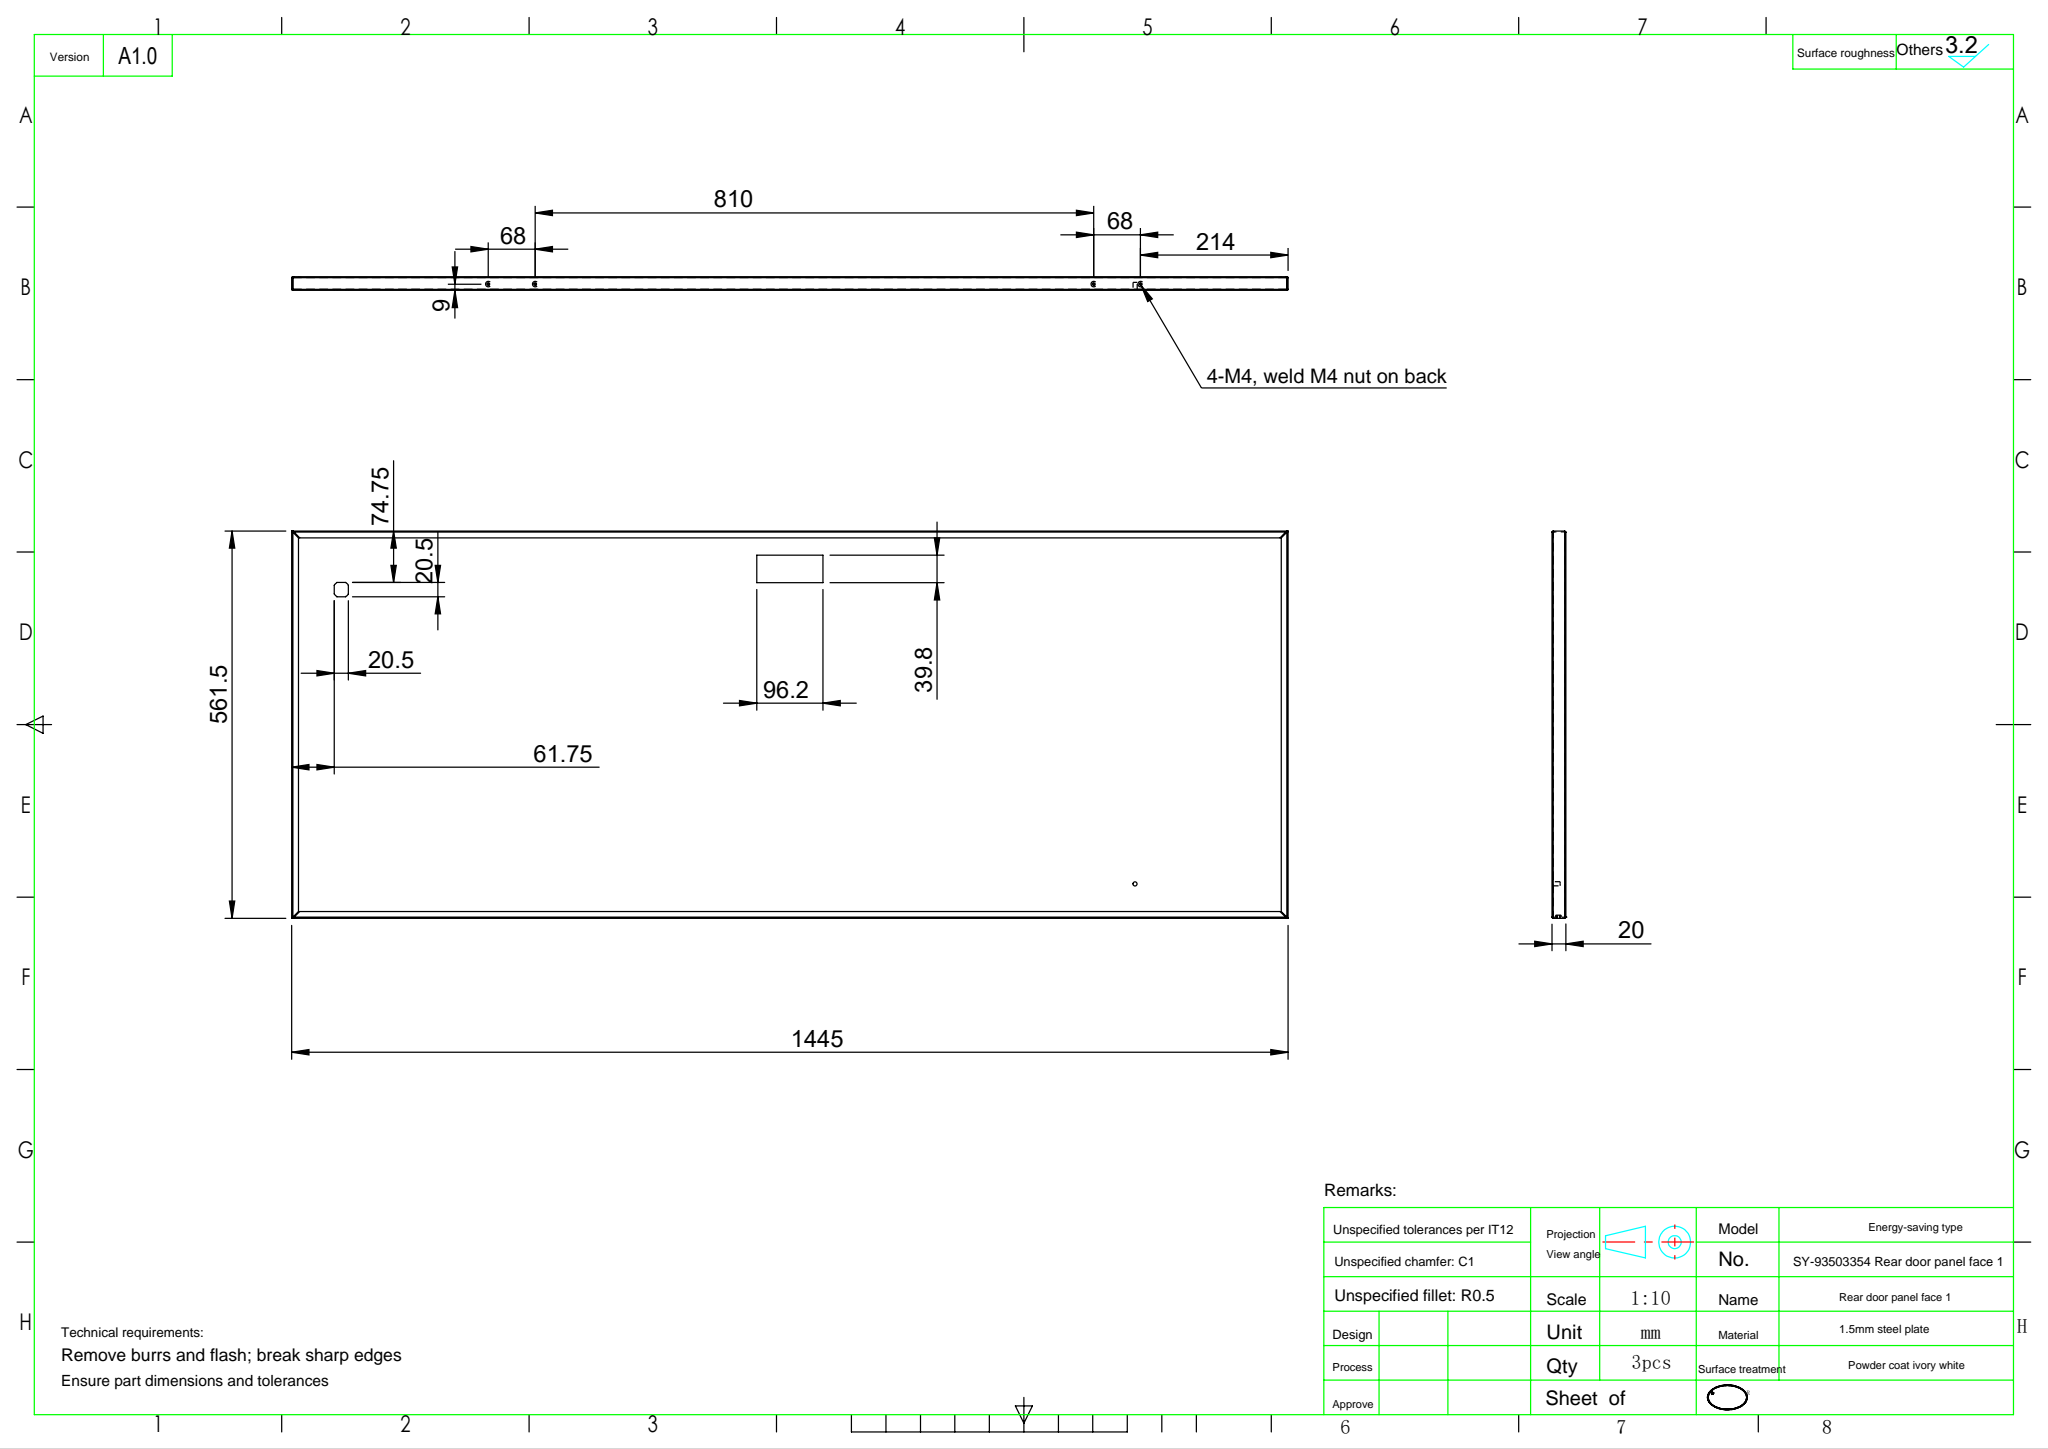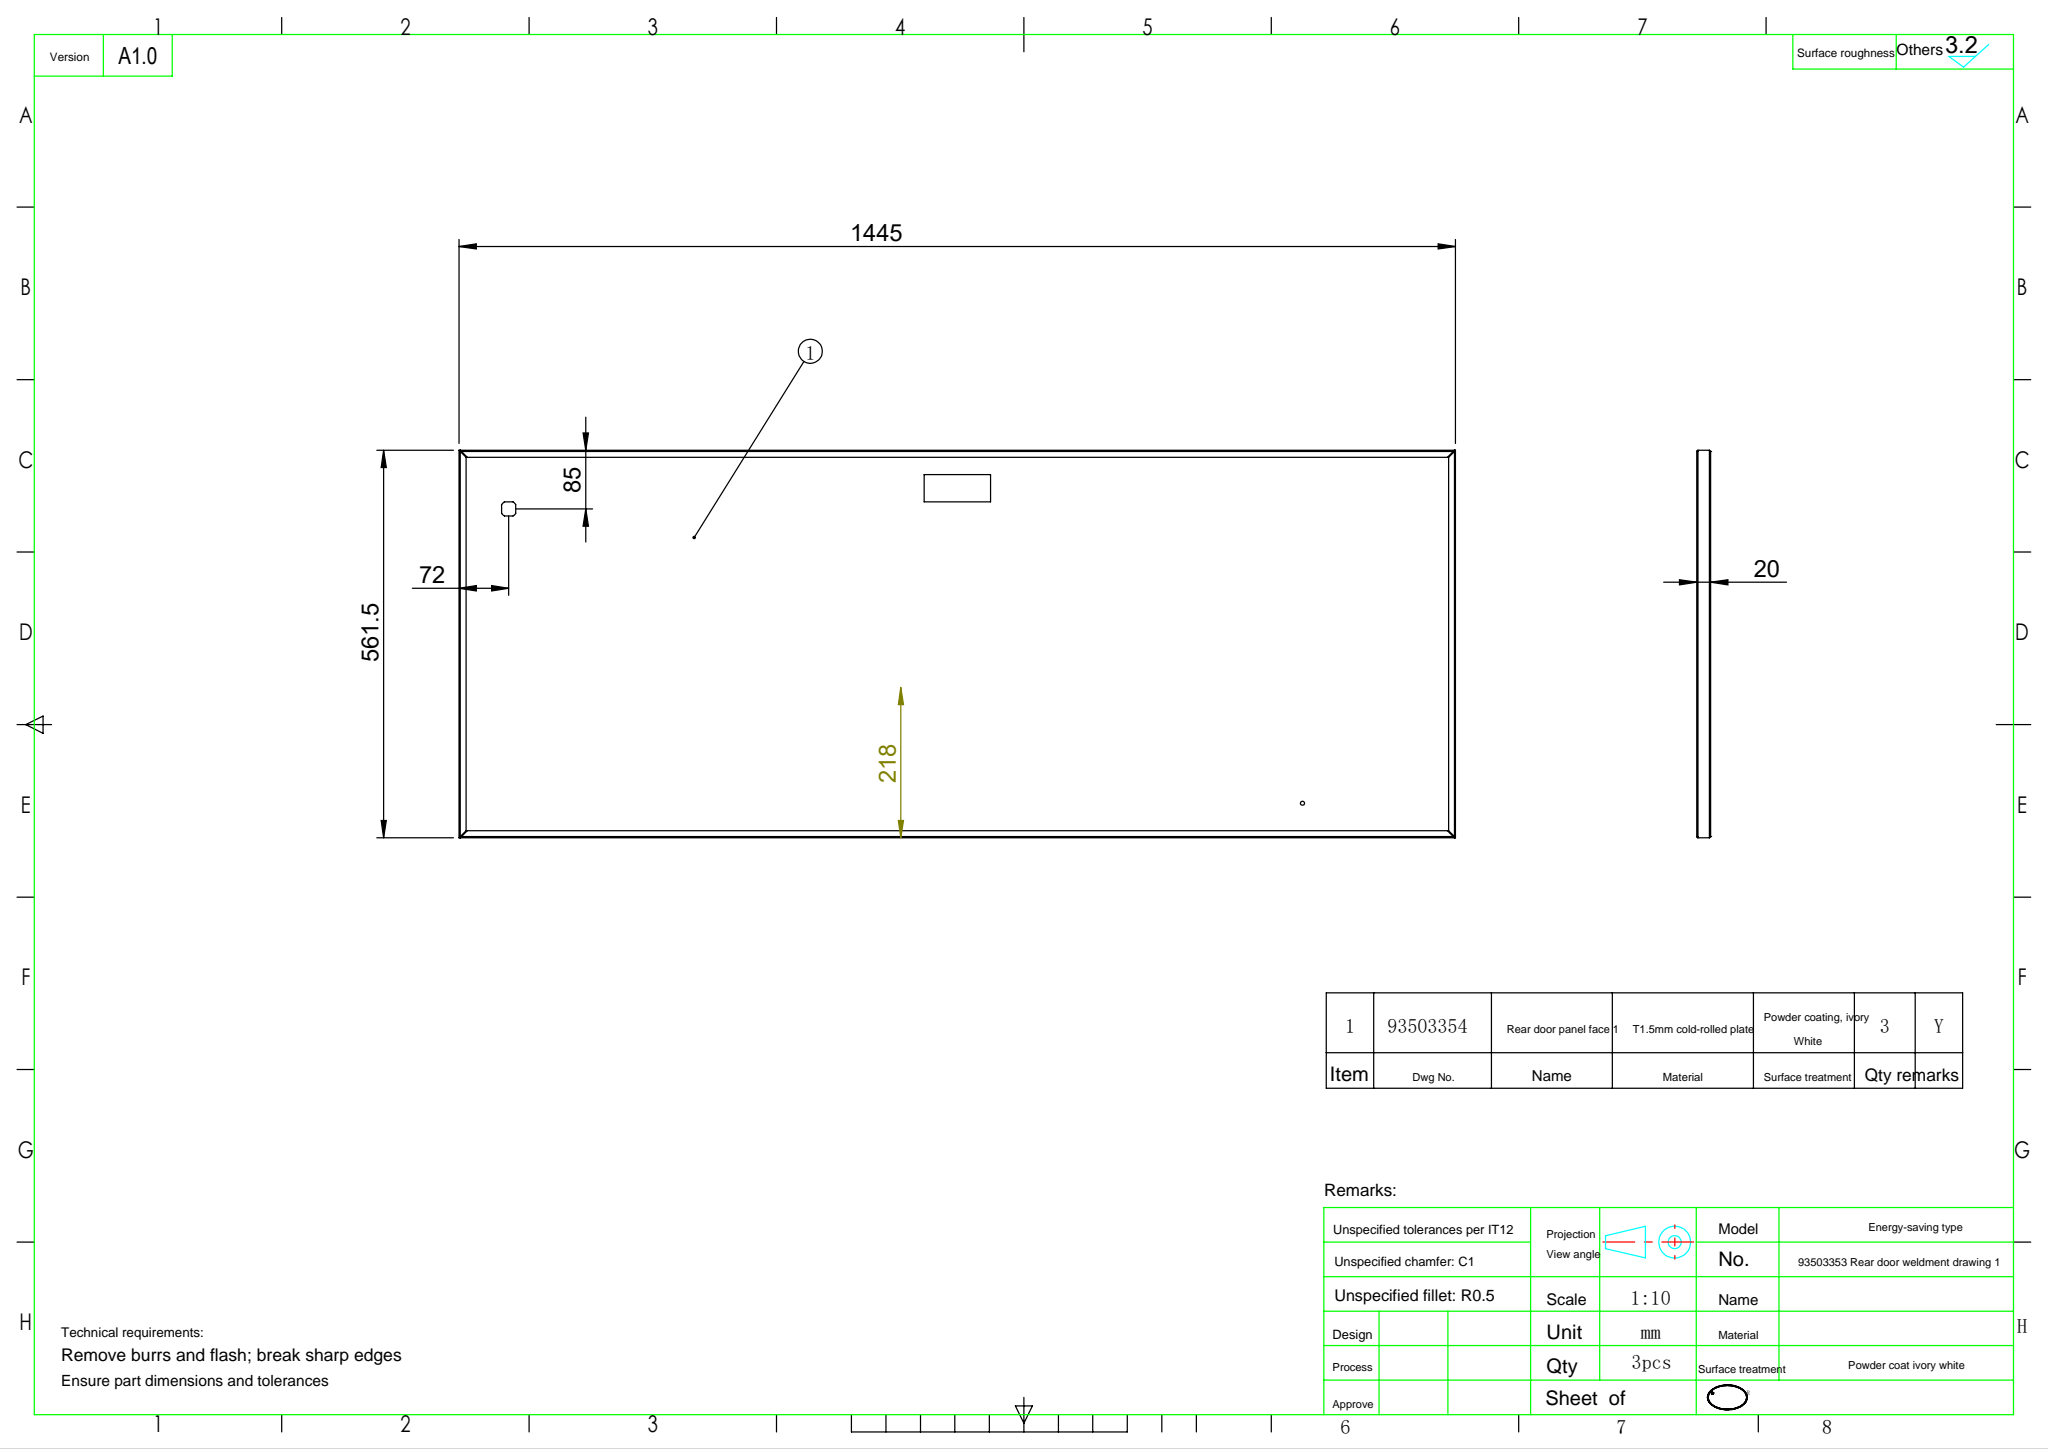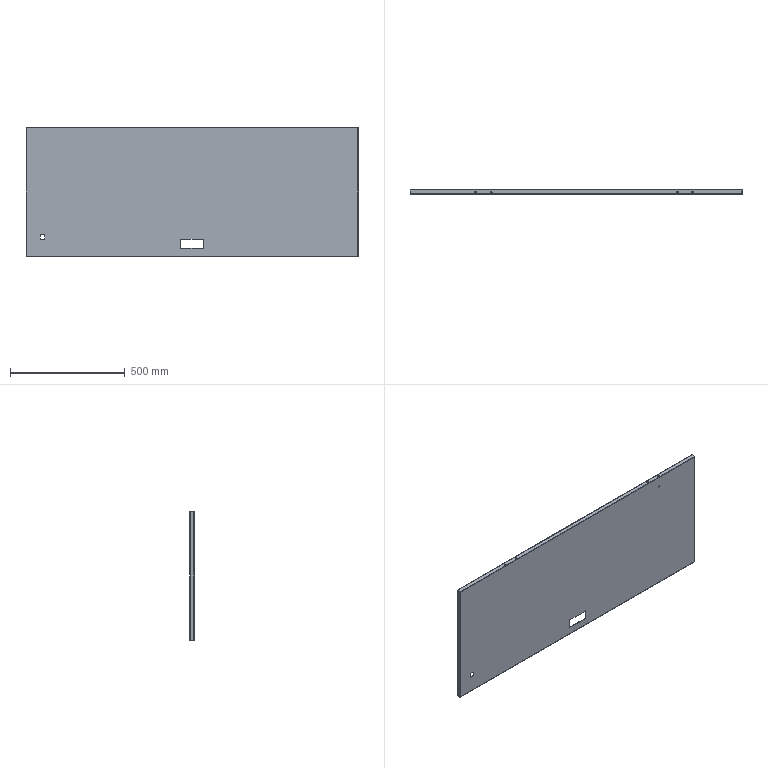Part | SolidWorks | features ICE 4, EdgeFlange 2, FlatPattern 1, HoleWzd 1, SMBaseFlange 1, SheetMetal 1 | 1 solid | 109 faces | box 1445 x 20 x 561.501 mm | volume 1368180 mm3 | plane 63 | cylinder 38 | spline 8 | commonest cylinder face diameters 0.4 x8 3.3 x8 3.4 x8 8 x8 24 x4 6 x2